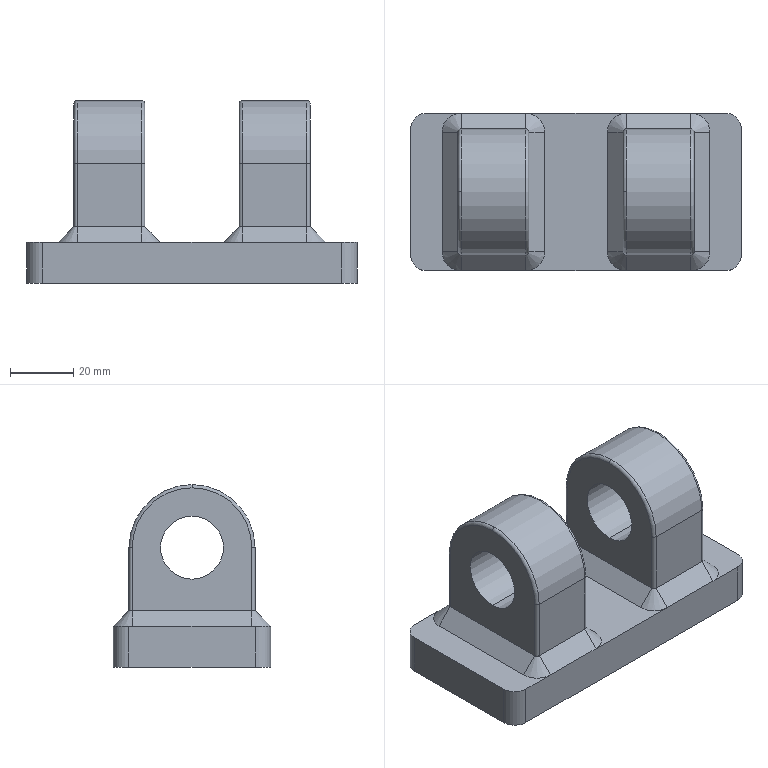Part | STEP file | Unit R-pair hinge lug | 1 solid | 56 faces | box 105 x 50 x 58 mm | volume 130356 mm3 | plane 24 | cylinder 18 | cone 8 | torus 6 | commonest cylinder face diameters 2 x8 10 x4 20 x4 40 x2